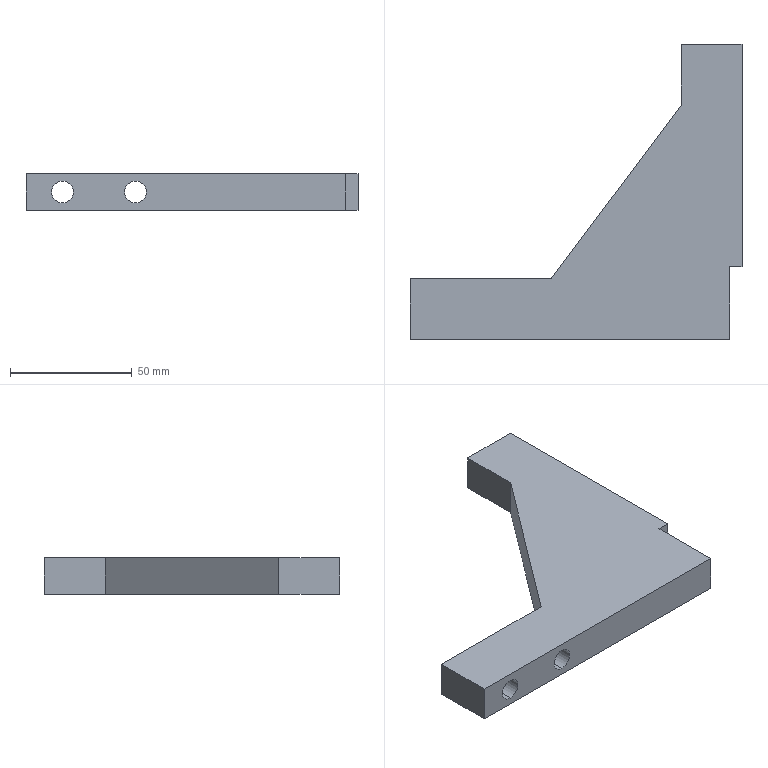Part | STEP file | 07-05 triangular support bracket | 1 solid | 27 faces | box 136.5 x 121.3 x 15 mm | volume 109879 mm3 | plane 11 | cylinder 10 | cone 6 | commonest cylinder face diameters 4.2 x6 9 x4
STEP:
#1=CARTESIAN_POINT('',(52.988,50.65,7.5));
#2=VERTEX_POINT('',#1);
#3=CARTESIAN_POINT('',(54.25,50.65,5.4));
#4=VERTEX_POINT('',#3);
#5=CARTESIAN_POINT('',(54.25,50.65,5.4));
#6=DIRECTION('',(0.515,0.,-0.8572));
#7=VECTOR('',#6,1000.);
#8=LINE('',#5,#7);
#9=EDGE_CURVE('',#2,#4,#8,.T.);
#10=ORIENTED_EDGE('',*,*,#9,.F.);
#11=CARTESIAN_POINT('',(54.25,50.65,9.6));
#12=VERTEX_POINT('',#11);
#13=CARTESIAN_POINT('',(54.25,50.65,9.6));
#14=DIRECTION('',(0.515,0.,0.8572));
#15=VECTOR('',#14,1000.);
#16=LINE('',#13,#15);
#17=EDGE_CURVE('',#2,#12,#16,.T.);
#18=ORIENTED_EDGE('',*,*,#17,.T.);
#19=CARTESIAN_POINT('',(54.25,50.65,7.5));
#20=DIRECTION('',(1.,0.,0.));
#21=DIRECTION('',(0.,0.,-1.));
#22=AXIS2_PLACEMENT_3D('',#19,#20,#21);
#23=CIRCLE('',#22,2.1);
#24=EDGE_CURVE('',#12,#4,#23,.T.);
#25=ORIENTED_EDGE('',*,*,#24,.T.);
#26=EDGE_LOOP('',(#10,#18,#25));
#27=FACE_OUTER_BOUND('',#26,.T.);
#28=CARTESIAN_POINT('',(54.25,50.65,7.5));
#29=DIRECTION('',(1.,0.,0.));
#30=DIRECTION('',(0.,0.,-1.));
#31=AXIS2_PLACEMENT_3D('',#28,#29,#30);
#32=CONICAL_SURFACE('',#31,2.1,1.03);
#33=ADVANCED_FACE('',(#27),#32,.F.);
#34=ORIENTED_EDGE('',*,*,#24,.F.);
#35=CARTESIAN_POINT('',(68.25,50.65,9.6));
#36=VERTEX_POINT('',#35);
#37=CARTESIAN_POINT('',(68.25,50.65,9.6));
#38=DIRECTION('',(1.,0.,0.));
#39=VECTOR('',#38,1000.);
#40=LINE('',#37,#39);
#41=EDGE_CURVE('',#12,#36,#40,.T.);
#42=ORIENTED_EDGE('',*,*,#41,.T.);
#43=CARTESIAN_POINT('',(68.25,50.65,5.4));
#44=VERTEX_POINT('',#43);
#45=CARTESIAN_POINT('',(68.25,50.65,7.5));
#46=DIRECTION('',(1.,0.,0.));
#47=DIRECTION('',(0.,0.,-1.));
#48=AXIS2_PLACEMENT_3D('',#45,#46,#47);
#49=CIRCLE('',#48,2.1);
#50=EDGE_CURVE('',#36,#44,#49,.T.);
#51=ORIENTED_EDGE('',*,*,#50,.T.);
#52=CARTESIAN_POINT('',(68.25,50.65,5.4));
#53=DIRECTION('',(1.,0.,0.));
#54=VECTOR('',#53,1000.);
#55=LINE('',#52,#54);
#56=EDGE_CURVE('',#4,#44,#55,.T.);
#57=ORIENTED_EDGE('',*,*,#56,.F.);
#58=EDGE_LOOP('',(#34,#42,#51,#57));
#59=FACE_OUTER_BOUND('',#58,.T.);
#60=CARTESIAN_POINT('',(68.25,50.65,7.5));
#61=DIRECTION('',(1.,0.,0.));
#62=DIRECTION('',(0.,0.,-1.));
#63=AXIS2_PLACEMENT_3D('',#60,#61,#62);
#64=CYLINDRICAL_SURFACE('',#63,2.1);
#65=ADVANCED_FACE('',(#59),#64,.F.);
#66=CARTESIAN_POINT('',(54.25,15.65,9.6));
#67=VERTEX_POINT('',#66);
#68=CARTESIAN_POINT('',(54.25,15.65,5.4));
#69=VERTEX_POINT('',#68);
#70=CARTESIAN_POINT('',(54.25,15.65,7.5));
#71=DIRECTION('',(1.,0.,0.));
#72=DIRECTION('',(0.,0.,-1.));
#73=AXIS2_PLACEMENT_3D('',#70,#71,#72);
#74=CIRCLE('',#73,2.1);
#75=EDGE_CURVE('',#67,#69,#74,.T.);
#76=ORIENTED_EDGE('',*,*,#75,.F.);
#77=CARTESIAN_POINT('',(68.25,15.65,9.6));
#78=VERTEX_POINT('',#77);
#79=CARTESIAN_POINT('',(68.25,15.65,9.6));
#80=DIRECTION('',(1.,0.,0.));
#81=VECTOR('',#80,1000.);
#82=LINE('',#79,#81);
#83=EDGE_CURVE('',#67,#78,#82,.T.);
#84=ORIENTED_EDGE('',*,*,#83,.T.);
#85=CARTESIAN_POINT('',(68.25,15.65,5.4));
#86=VERTEX_POINT('',#85);
#87=CARTESIAN_POINT('',(68.25,15.65,7.5));
#88=DIRECTION('',(1.,0.,0.));
#89=DIRECTION('',(0.,0.,-1.));
#90=AXIS2_PLACEMENT_3D('',#87,#88,#89);
#91=CIRCLE('',#90,2.1);
#92=EDGE_CURVE('',#78,#86,#91,.T.);
#93=ORIENTED_EDGE('',*,*,#92,.T.);
#94=CARTESIAN_POINT('',(68.25,15.65,5.4));
#95=DIRECTION('',(1.,0.,0.));
#96=VECTOR('',#95,1000.);
#97=LINE('',#94,#96);
#98=EDGE_CURVE('',#69,#86,#97,.T.);
#99=ORIENTED_EDGE('',*,*,#98,.F.);
#100=EDGE_LOOP('',(#76,#84,#93,#99));
#101=FACE_OUTER_BOUND('',#100,.T.);
#102=CARTESIAN_POINT('',(68.25,15.65,7.5));
#103=DIRECTION('',(1.,0.,0.));
#104=DIRECTION('',(0.,0.,-1.));
#105=AXIS2_PLACEMENT_3D('',#102,#103,#104);
#106=CYLINDRICAL_SURFACE('',#105,2.1);
#107=ADVANCED_FACE('',(#101),#106,.F.);
#108=CARTESIAN_POINT('',(52.988,15.65,7.5));
#109=VERTEX_POINT('',#108);
#110=CARTESIAN_POINT('',(54.25,15.65,5.4));
#111=DIRECTION('',(0.515,0.,-0.8572));
#112=VECTOR('',#111,1000.);
#113=LINE('',#110,#112);
#114=EDGE_CURVE('',#109,#69,#113,.T.);
#115=ORIENTED_EDGE('',*,*,#114,.F.);
#116=CARTESIAN_POINT('',(54.25,15.65,9.6));
#117=DIRECTION('',(0.515,0.,0.8572));
#118=VECTOR('',#117,1000.);
#119=LINE('',#116,#118);
#120=EDGE_CURVE('',#109,#67,#119,.T.);
#121=ORIENTED_EDGE('',*,*,#120,.T.);
#122=ORIENTED_EDGE('',*,*,#75,.T.);
#123=EDGE_LOOP('',(#115,#121,#122));
#124=FACE_OUTER_BOUND('',#123,.T.);
#125=CARTESIAN_POINT('',(54.25,15.65,7.5));
#126=DIRECTION('',(1.,0.,0.));
#127=DIRECTION('',(0.,0.,-1.));
#128=AXIS2_PLACEMENT_3D('',#125,#126,#127);
#129=CONICAL_SURFACE('',#128,2.1,1.03);
#130=ADVANCED_FACE('',(#124),#129,.F.);
#131=CARTESIAN_POINT('',(54.25,-19.35,9.6));
#132=VERTEX_POINT('',#131);
#133=CARTESIAN_POINT('',(54.25,-19.35,5.4));
#134=VERTEX_POINT('',#133);
#135=CARTESIAN_POINT('',(54.25,-19.35,7.5));
#136=DIRECTION('',(1.,0.,0.));
#137=DIRECTION('',(0.,0.,-1.));
#138=AXIS2_PLACEMENT_3D('',#135,#136,#137);
#139=CIRCLE('',#138,2.1);
#140=EDGE_CURVE('',#132,#134,#139,.T.);
#141=ORIENTED_EDGE('',*,*,#140,.F.);
#142=CARTESIAN_POINT('',(68.25,-19.35,9.6));
#143=VERTEX_POINT('',#142);
#144=CARTESIAN_POINT('',(68.25,-19.35,9.6));
#145=DIRECTION('',(1.,0.,0.));
#146=VECTOR('',#145,1000.);
#147=LINE('',#144,#146);
#148=EDGE_CURVE('',#132,#143,#147,.T.);
#149=ORIENTED_EDGE('',*,*,#148,.T.);
#150=CARTESIAN_POINT('',(68.25,-19.35,5.4));
#151=VERTEX_POINT('',#150);
#152=CARTESIAN_POINT('',(68.25,-19.35,7.5));
#153=DIRECTION('',(1.,0.,0.));
#154=DIRECTION('',(0.,0.,-1.));
#155=AXIS2_PLACEMENT_3D('',#152,#153,#154);
#156=CIRCLE('',#155,2.1);
#157=EDGE_CURVE('',#143,#151,#156,.T.);
#158=ORIENTED_EDGE('',*,*,#157,.T.);
#159=CARTESIAN_POINT('',(68.25,-19.35,5.4));
#160=DIRECTION('',(1.,0.,0.));
#161=VECTOR('',#160,1000.);
#162=LINE('',#159,#161);
#163=EDGE_CURVE('',#134,#151,#162,.T.);
#164=ORIENTED_EDGE('',*,*,#163,.F.);
#165=EDGE_LOOP('',(#141,#149,#158,#164));
#166=FACE_OUTER_BOUND('',#165,.T.);
#167=CARTESIAN_POINT('',(68.25,-19.35,7.5));
#168=DIRECTION('',(1.,0.,0.));
#169=DIRECTION('',(0.,0.,-1.));
#170=AXIS2_PLACEMENT_3D('',#167,#168,#169);
#171=CYLINDRICAL_SURFACE('',#170,2.1);
#172=ADVANCED_FACE('',(#166),#171,.F.);
#173=CARTESIAN_POINT('',(52.988,-19.35,7.5));
#174=VERTEX_POINT('',#173);
#175=CARTESIAN_POINT('',(54.25,-19.35,5.4));
#176=DIRECTION('',(0.515,0.,-0.8572));
#177=VECTOR('',#176,1000.);
#178=LINE('',#175,#177);
#179=EDGE_CURVE('',#174,#134,#178,.T.);
#180=ORIENTED_EDGE('',*,*,#179,.F.);
#181=CARTESIAN_POINT('',(54.25,-19.35,9.6));
#182=DIRECTION('',(0.515,0.,0.8572));
#183=VECTOR('',#182,1000.);
#184=LINE('',#181,#183);
#185=EDGE_CURVE('',#174,#132,#184,.T.);
#186=ORIENTED_EDGE('',*,*,#185,.T.);
#187=ORIENTED_EDGE('',*,*,#140,.T.);
#188=EDGE_LOOP('',(#180,#186,#187));
#189=FACE_OUTER_BOUND('',#188,.T.);
#190=CARTESIAN_POINT('',(54.25,-19.35,7.5));
#191=DIRECTION('',(1.,0.,0.));
#192=DIRECTION('',(0.,0.,-1.));
#193=AXIS2_PLACEMENT_3D('',#190,#191,#192);
#194=CONICAL_SURFACE('',#193,2.1,1.03);
#195=ADVANCED_FACE('',(#189),#194,.F.);
#196=CARTESIAN_POINT('',(-23.25,-60.65,3.));
#197=VERTEX_POINT('',#196);
#198=CARTESIAN_POINT('',(-23.25,-60.65,12.));
#199=VERTEX_POINT('',#198);
#200=CARTESIAN_POINT('',(-23.25,-60.65,7.5));
#201=DIRECTION('',(0.,1.,0.));
#202=DIRECTION('',(0.,0.,1.));
#203=AXIS2_PLACEMENT_3D('',#200,#201,#202);
#204=CIRCLE('',#203,4.5);
#205=EDGE_CURVE('',#197,#199,#204,.T.);
#206=ORIENTED_EDGE('',*,*,#205,.F.);
#207=CARTESIAN_POINT('',(-23.25,-35.65,3.));
#208=VERTEX_POINT('',#207);
#209=CARTESIAN_POINT('',(-23.25,-65.65,3.));
#210=DIRECTION('',(0.,1.,0.));
#211=VECTOR('',#210,1000.);
#212=LINE('',#209,#211);
#213=EDGE_CURVE('',#197,#208,#212,.T.);
#214=ORIENTED_EDGE('',*,*,#213,.T.);
#215=CARTESIAN_POINT('',(-23.25,-35.65,12.));
#216=VERTEX_POINT('',#215);
#217=CARTESIAN_POINT('',(-23.25,-35.65,7.5));
#218=DIRECTION('',(0.,-1.,0.));
#219=DIRECTION('',(0.,0.,-1.));
#220=AXIS2_PLACEMENT_3D('',#217,#218,#219);
#221=CIRCLE('',#220,4.5);
#222=EDGE_CURVE('',#216,#208,#221,.T.);
#223=ORIENTED_EDGE('',*,*,#222,.F.);
#224=CARTESIAN_POINT('',(-23.25,-65.65,12.));
#225=DIRECTION('',(0.,1.,0.));
#226=VECTOR('',#225,1000.);
#227=LINE('',#224,#226);
#228=EDGE_CURVE('',#199,#216,#227,.T.);
#229=ORIENTED_EDGE('',*,*,#228,.F.);
#230=EDGE_LOOP('',(#206,#214,#223,#229));
#231=FACE_OUTER_BOUND('',#230,.T.);
#232=CARTESIAN_POINT('',(-23.25,-65.65,7.5));
#233=DIRECTION('',(0.,1.,0.));
#234=DIRECTION('',(0.,0.,1.));
#235=AXIS2_PLACEMENT_3D('',#232,#233,#234);
#236=CYLINDRICAL_SURFACE('',#235,4.5);
#237=ADVANCED_FACE('',(#231),#236,.F.);
#238=CARTESIAN_POINT('',(-53.25,-60.65,3.));
#239=VERTEX_POINT('',#238);
#240=CARTESIAN_POINT('',(-53.25,-60.65,12.));
#241=VERTEX_POINT('',#240);
#242=CARTESIAN_POINT('',(-53.25,-60.65,7.5));
#243=DIRECTION('',(0.,1.,0.));
#244=DIRECTION('',(0.,0.,1.));
#245=AXIS2_PLACEMENT_3D('',#242,#243,#244);
#246=CIRCLE('',#245,4.5);
#247=EDGE_CURVE('',#239,#241,#246,.T.);
#248=ORIENTED_EDGE('',*,*,#247,.F.);
#249=CARTESIAN_POINT('',(-53.25,-35.65,3.));
#250=VERTEX_POINT('',#249);
#251=CARTESIAN_POINT('',(-53.25,-65.65,3.));
#252=DIRECTION('',(0.,1.,0.));
#253=VECTOR('',#252,1000.);
#254=LINE('',#251,#253);
#255=EDGE_CURVE('',#239,#250,#254,.T.);
#256=ORIENTED_EDGE('',*,*,#255,.T.);
#257=CARTESIAN_POINT('',(-53.25,-35.65,12.));
#258=VERTEX_POINT('',#257);
#259=CARTESIAN_POINT('',(-53.25,-35.65,7.5));
#260=DIRECTION('',(0.,-1.,0.));
#261=DIRECTION('',(0.,0.,-1.));
#262=AXIS2_PLACEMENT_3D('',#259,#260,#261);
#263=CIRCLE('',#262,4.5);
#264=EDGE_CURVE('',#258,#250,#263,.T.);
#265=ORIENTED_EDGE('',*,*,#264,.F.);
#266=CARTESIAN_POINT('',(-53.25,-65.65,12.));
#267=DIRECTION('',(0.,1.,0.));
#268=VECTOR('',#267,1000.);
#269=LINE('',#266,#268);
#270=EDGE_CURVE('',#241,#258,#269,.T.);
#271=ORIENTED_EDGE('',*,*,#270,.F.);
#272=EDGE_LOOP('',(#248,#256,#265,#271));
#273=FACE_OUTER_BOUND('',#272,.T.);
#274=CARTESIAN_POINT('',(-53.25,-65.65,7.5));
#275=DIRECTION('',(0.,1.,0.));
#276=DIRECTION('',(0.,0.,1.));
#277=AXIS2_PLACEMENT_3D('',#274,#275,#276);
#278=CYLINDRICAL_SURFACE('',#277,4.5);
#279=ADVANCED_FACE('',(#273),#278,.F.);
#280=CARTESIAN_POINT('',(68.25,15.65,7.5));
#281=DIRECTION('',(1.,0.,0.));
#282=DIRECTION('',(0.,0.,-1.));
#283=AXIS2_PLACEMENT_3D('',#280,#281,#282);
#284=CIRCLE('',#283,2.1);
#285=EDGE_CURVE('',#86,#78,#284,.T.);
#286=ORIENTED_EDGE('',*,*,#285,.F.);
#287=ORIENTED_EDGE('',*,*,#92,.F.);
#288=EDGE_LOOP('',(#286,#287));
#289=FACE_BOUND('',#288,.T.);
#290=CARTESIAN_POINT('',(68.25,-19.35,7.5));
#291=DIRECTION('',(1.,0.,0.));
#292=DIRECTION('',(0.,0.,-1.));
#293=AXIS2_PLACEMENT_3D('',#290,#291,#292);
#294=CIRCLE('',#293,2.1);
#295=EDGE_CURVE('',#151,#143,#294,.T.);
#296=ORIENTED_EDGE('',*,*,#295,.F.);
#297=ORIENTED_EDGE('',*,*,#157,.F.);
#298=EDGE_LOOP('',(#296,#297));
#299=FACE_BOUND('',#298,.T.);
#300=CARTESIAN_POINT('',(68.25,-30.65,15.));
#301=VERTEX_POINT('',#300);
#302=CARTESIAN_POINT('',(68.25,60.65,15.));
#303=VERTEX_POINT('',#302);
#304=CARTESIAN_POINT('',(68.25,-60.65,15.));
#305=DIRECTION('',(0.,1.,0.));
#306=VECTOR('',#305,1000.);
#307=LINE('',#304,#306);
#308=EDGE_CURVE('',#301,#303,#307,.T.);
#309=ORIENTED_EDGE('',*,*,#308,.F.);
#310=CARTESIAN_POINT('',(68.25,-30.65,0.));
#311=VERTEX_POINT('',#310);
#312=CARTESIAN_POINT('',(68.25,-30.65,-83.));
#313=DIRECTION('',(0.,0.,1.));
#314=VECTOR('',#313,1000.);
#315=LINE('',#312,#314);
#316=EDGE_CURVE('',#311,#301,#315,.T.);
#317=ORIENTED_EDGE('',*,*,#316,.F.);
#318=CARTESIAN_POINT('',(68.25,60.65,0.));
#319=VERTEX_POINT('',#318);
#320=CARTESIAN_POINT('',(68.25,-60.65,0.));
#321=DIRECTION('',(0.,1.,0.));
#322=VECTOR('',#321,1000.);
#323=LINE('',#320,#322);
#324=EDGE_CURVE('',#311,#319,#323,.T.);
#325=ORIENTED_EDGE('',*,*,#324,.T.);
#326=CARTESIAN_POINT('',(68.25,60.65,15.));
#327=DIRECTION('',(0.,0.,-1.));
#328=VECTOR('',#327,1000.);
#329=LINE('',#326,#328);
#330=EDGE_CURVE('',#303,#319,#329,.T.);
#331=ORIENTED_EDGE('',*,*,#330,.F.);
#332=EDGE_LOOP('',(#309,#317,#325,#331));
#333=FACE_OUTER_BOUND('',#332,.T.);
#334=CARTESIAN_POINT('',(68.25,50.65,7.5));
#335=DIRECTION('',(1.,0.,0.));
#336=DIRECTION('',(0.,0.,-1.));
#337=AXIS2_PLACEMENT_3D('',#334,#335,#336);
#338=CIRCLE('',#337,2.1);
#339=EDGE_CURVE('',#44,#36,#338,.T.);
#340=ORIENTED_EDGE('',*,*,#339,.F.);
#341=ORIENTED_EDGE('',*,*,#50,.F.);
#342=EDGE_LOOP('',(#340,#341));
#343=FACE_BOUND('',#342,.T.);
#344=CARTESIAN_POINT('',(68.25,-60.65,15.));
#345=DIRECTION('',(-1.,0.,0.));
#346=DIRECTION('',(0.,0.,1.));
#347=AXIS2_PLACEMENT_3D('',#344,#345,#346);
#348=PLANE('',#347);
#349=ADVANCED_FACE('',(#289,#299,#333,#343),#348,.F.);
#350=CARTESIAN_POINT('',(43.25,60.65,0.));
#351=VERTEX_POINT('',#350);
#352=CARTESIAN_POINT('',(-68.25,60.65,0.));
#353=DIRECTION('',(-1.,0.,0.));
#354=VECTOR('',#353,1000.);
#355=LINE('',#352,#354);
#356=EDGE_CURVE('',#319,#351,#355,.T.);
#357=ORIENTED_EDGE('',*,*,#356,.T.);
#358=CARTESIAN_POINT('',(43.25,60.65,15.));
#359=VERTEX_POINT('',#358);
#360=CARTESIAN_POINT('',(43.25,60.65,-33.));
#361=DIRECTION('',(0.,0.,1.));
#362=VECTOR('',#361,1000.);
#363=LINE('',#360,#362);
#364=EDGE_CURVE('',#351,#359,#363,.T.);
#365=ORIENTED_EDGE('',*,*,#364,.T.);
#366=CARTESIAN_POINT('',(-68.25,60.65,15.));
#367=DIRECTION('',(-1.,0.,0.));
#368=VECTOR('',#367,1000.);
#369=LINE('',#366,#368);
#370=EDGE_CURVE('',#303,#359,#369,.T.);
#371=ORIENTED_EDGE('',*,*,#370,.F.);
#372=ORIENTED_EDGE('',*,*,#330,.T.);
#373=EDGE_LOOP('',(#357,#365,#371,#372));
#374=FACE_OUTER_BOUND('',#373,.T.);
#375=CARTESIAN_POINT('',(-68.25,60.65,15.));
#376=DIRECTION('',(0.,-1.,0.));
#377=DIRECTION('',(0.,0.,-1.));
#378=AXIS2_PLACEMENT_3D('',#375,#376,#377);
#379=PLANE('',#378);
#380=ADVANCED_FACE('',(#374),#379,.F.);
#381=CARTESIAN_POINT('',(-68.25,-35.65,15.));
#382=VERTEX_POINT('',#381);
#383=CARTESIAN_POINT('',(-68.25,-60.65,15.));
#384=VERTEX_POINT('',#383);
#385=CARTESIAN_POINT('',(-68.25,-60.65,15.));
#386=DIRECTION('',(0.,-1.,0.));
#387=VECTOR('',#386,1000.);
#388=LINE('',#385,#387);
#389=EDGE_CURVE('',#382,#384,#388,.T.);
#390=ORIENTED_EDGE('',*,*,#389,.F.);
#391=CARTESIAN_POINT('',(-68.25,-35.65,0.));
#392=VERTEX_POINT('',#391);
#393=CARTESIAN_POINT('',(-68.25,-35.65,-33.));
#394=DIRECTION('',(0.,0.,1.));
#395=VECTOR('',#394,1000.);
#396=LINE('',#393,#395);
#397=EDGE_CURVE('',#392,#382,#396,.T.);
#398=ORIENTED_EDGE('',*,*,#397,.F.);
#399=CARTESIAN_POINT('',(-68.25,-60.65,0.));
#400=VERTEX_POINT('',#399);
#401=CARTESIAN_POINT('',(-68.25,-60.65,0.));
#402=DIRECTION('',(0.,-1.,0.));
#403=VECTOR('',#402,1000.);
#404=LINE('',#401,#403);
#405=EDGE_CURVE('',#392,#400,#404,.T.);
#406=ORIENTED_EDGE('',*,*,#405,.T.);
#407=CARTESIAN_POINT('',(-68.25,-60.65,15.));
#408=DIRECTION('',(0.,0.,-1.));
#409=VECTOR('',#408,1000.);
#410=LINE('',#407,#409);
#411=EDGE_CURVE('',#384,#400,#410,.T.);
#412=ORIENTED_EDGE('',*,*,#411,.F.);
#413=EDGE_LOOP('',(#390,#398,#406,#412));
#414=FACE_OUTER_BOUND('',#413,.T.);
#415=CARTESIAN_POINT('',(-68.25,-60.65,15.));
#416=DIRECTION('',(1.,0.,0.));
#417=DIRECTION('',(0.,0.,-1.));
#418=AXIS2_PLACEMENT_3D('',#415,#416,#417);
#419=PLANE('',#418);
#420=ADVANCED_FACE('',(#414),#419,.F.);
#421=CARTESIAN_POINT('',(-23.25,-60.65,7.5));
#422=DIRECTION('',(0.,1.,0.));
#423=DIRECTION('',(0.,0.,1.));
#424=AXIS2_PLACEMENT_3D('',#421,#422,#423);
#425=CIRCLE('',#424,4.5);
#426=EDGE_CURVE('',#199,#197,#425,.T.);
#427=ORIENTED_EDGE('',*,*,#426,.T.);
#428=ORIENTED_EDGE('',*,*,#205,.T.);
#429=EDGE_LOOP('',(#427,#428));
#430=FACE_BOUND('',#429,.T.);
#431=CARTESIAN_POINT('',(-53.25,-60.65,7.5));
#432=DIRECTION('',(0.,1.,0.));
#433=DIRECTION('',(0.,0.,1.));
#434=AXIS2_PLACEMENT_3D('',#431,#432,#433);
#435=CIRCLE('',#434,4.5);
#436=EDGE_CURVE('',#241,#239,#435,.T.);
#437=ORIENTED_EDGE('',*,*,#436,.T.);
#438=ORIENTED_EDGE('',*,*,#247,.T.);
#439=EDGE_LOOP('',(#437,#438));
#440=FACE_BOUND('',#439,.T.);
#441=CARTESIAN_POINT('',(63.25,-60.65,0.));
#442=VERTEX_POINT('',#441);
#443=CARTESIAN_POINT('',(-68.25,-60.65,0.));
#444=DIRECTION('',(1.,0.,0.));
#445=VECTOR('',#444,1000.);
#446=LINE('',#443,#445);
#447=EDGE_CURVE('',#400,#442,#446,.T.);
#448=ORIENTED_EDGE('',*,*,#447,.T.);
#449=CARTESIAN_POINT('',(63.25,-60.65,15.));
#450=VERTEX_POINT('',#449);
#451=CARTESIAN_POINT('',(63.25,-60.65,-83.));
#452=DIRECTION('',(0.,0.,1.));
#453=VECTOR('',#452,1000.);
#454=LINE('',#451,#453);
#455=EDGE_CURVE('',#442,#450,#454,.T.);
#456=ORIENTED_EDGE('',*,*,#455,.T.);
#457=CARTESIAN_POINT('',(-68.25,-60.65,15.));
#458=DIRECTION('',(1.,0.,0.));
#459=VECTOR('',#458,1000.);
#460=LINE('',#457,#459);
#461=EDGE_CURVE('',#384,#450,#460,.T.);
#462=ORIENTED_EDGE('',*,*,#461,.F.);
#463=ORIENTED_EDGE('',*,*,#411,.T.);
#464=EDGE_LOOP('',(#448,#456,#462,#463));
#465=FACE_OUTER_BOUND('',#464,.T.);
#466=CARTESIAN_POINT('',(-68.25,-60.65,15.));
#467=DIRECTION('',(0.,1.,0.));
#468=DIRECTION('',(0.,0.,1.));
#469=AXIS2_PLACEMENT_3D('',#466,#467,#468);
#470=PLANE('',#469);
#471=ADVANCED_FACE('',(#430,#440,#465),#470,.F.);
#472=ORIENTED_EDGE('',*,*,#461,.T.);
#473=CARTESIAN_POINT('',(63.25,-30.65,15.));
#474=VERTEX_POINT('',#473);
#475=CARTESIAN_POINT('',(63.25,-60.65,15.));
#476=DIRECTION('',(0.,-1.,0.));
#477=VECTOR('',#476,1000.);
#478=LINE('',#475,#477);
#479=EDGE_CURVE('',#474,#450,#478,.T.);
#480=ORIENTED_EDGE('',*,*,#479,.F.);
#481=CARTESIAN_POINT('',(68.25,-30.65,15.));
#482=DIRECTION('',(-1.,0.,0.));
#483=VECTOR('',#482,1000.);
#484=LINE('',#481,#483);
#485=EDGE_CURVE('',#301,#474,#484,.T.);
#486=ORIENTED_EDGE('',*,*,#485,.F.);
#487=ORIENTED_EDGE('',*,*,#308,.T.);
#488=ORIENTED_EDGE('',*,*,#370,.T.);
#489=CARTESIAN_POINT('',(43.25,35.65,15.));
#490=VERTEX_POINT('',#489);
#491=CARTESIAN_POINT('',(43.25,60.65,15.));
#492=DIRECTION('',(0.,1.,0.));
#493=VECTOR('',#492,1000.);
#494=LINE('',#491,#493);
#495=EDGE_CURVE('',#490,#359,#494,.T.);
#496=ORIENTED_EDGE('',*,*,#495,.F.);
#497=CARTESIAN_POINT('',(-10.25,-35.65,15.));
#498=VERTEX_POINT('',#497);
#499=CARTESIAN_POINT('',(43.25,35.65,15.));
#500=DIRECTION('',(0.6002,0.7999,0.));
#501=VECTOR('',#500,1000.);
#502=LINE('',#499,#501);
#503=EDGE_CURVE('',#498,#490,#502,.T.);
#504=ORIENTED_EDGE('',*,*,#503,.F.);
#505=CARTESIAN_POINT('',(-68.25,-35.65,15.));
#506=DIRECTION('',(1.,0.,0.));
#507=VECTOR('',#506,1000.);
#508=LINE('',#505,#507);
#509=EDGE_CURVE('',#382,#498,#508,.T.);
#510=ORIENTED_EDGE('',*,*,#509,.F.);
#511=ORIENTED_EDGE('',*,*,#389,.T.);
#512=EDGE_LOOP('',(#472,#480,#486,#487,#488,#496,#504,#510,#511));
#513=FACE_OUTER_BOUND('',#512,.T.);
#514=CARTESIAN_POINT('',(68.25,60.65,15.));
#515=DIRECTION('',(0.,0.,-1.));
#516=DIRECTION('',(-1.,0.,0.));
#517=AXIS2_PLACEMENT_3D('',#514,#515,#516);
#518=PLANE('',#517);
#519=ADVANCED_FACE('',(#513),#518,.F.);
#520=CARTESIAN_POINT('',(63.25,-30.65,0.));
#521=VERTEX_POINT('',#520);
#522=CARTESIAN_POINT('',(63.25,60.65,0.));
#523=DIRECTION('',(0.,1.,0.));
#524=VECTOR('',#523,1000.);
#525=LINE('',#522,#524);
#526=EDGE_CURVE('',#442,#521,#525,.T.);
#527=ORIENTED_EDGE('',*,*,#526,.F.);
#528=ORIENTED_EDGE('',*,*,#447,.F.);
#529=ORIENTED_EDGE('',*,*,#405,.F.);
#530=CARTESIAN_POINT('',(-10.25,-35.65,0.));
#531=VERTEX_POINT('',#530);
#532=CARTESIAN_POINT('',(68.25,-35.65,0.));
#533=DIRECTION('',(-1.,0.,0.));
#534=VECTOR('',#533,1000.);
#535=LINE('',#532,#534);
#536=EDGE_CURVE('',#531,#392,#535,.T.);
#537=ORIENTED_EDGE('',*,*,#536,.F.);
#538=CARTESIAN_POINT('',(43.25,35.65,0.));
#539=VERTEX_POINT('',#538);
#540=CARTESIAN_POINT('',(64.257,63.646,0.));
#541=DIRECTION('',(-0.6002,-0.7999,0.));
#542=VECTOR('',#541,1000.);
#543=LINE('',#540,#542);
#544=EDGE_CURVE('',#539,#531,#543,.T.);
#545=ORIENTED_EDGE('',*,*,#544,.F.);
#546=CARTESIAN_POINT('',(43.25,60.65,0.));
#547=DIRECTION('',(0.,-1.,0.));
#548=VECTOR('',#547,1000.);
#549=LINE('',#546,#548);
#550=EDGE_CURVE('',#351,#539,#549,.T.);
#551=ORIENTED_EDGE('',*,*,#550,.F.);
#552=ORIENTED_EDGE('',*,*,#356,.F.);
#553=ORIENTED_EDGE('',*,*,#324,.F.);
#554=CARTESIAN_POINT('',(68.25,-30.65,0.));
#555=DIRECTION('',(1.,0.,0.));
#556=VECTOR('',#555,1000.);
#557=LINE('',#554,#556);
#558=EDGE_CURVE('',#521,#311,#557,.T.);
#559=ORIENTED_EDGE('',*,*,#558,.F.);
#560=EDGE_LOOP('',(#527,#528,#529,#537,#545,#551,#552,#553,#559));
#561=FACE_OUTER_BOUND('',#560,.T.);
#562=CARTESIAN_POINT('',(68.25,60.65,0.));
#563=DIRECTION('',(0.,0.,-1.));
#564=DIRECTION('',(-1.,0.,0.));
#565=AXIS2_PLACEMENT_3D('',#562,#563,#564);
#566=PLANE('',#565);
#567=ADVANCED_FACE('',(#561),#566,.T.);
#568=ORIENTED_EDGE('',*,*,#550,.T.);
#569=CARTESIAN_POINT('',(43.25,35.65,-33.));
#570=DIRECTION('',(0.,0.,1.));
#571=VECTOR('',#570,1000.);
#572=LINE('',#569,#571);
#573=EDGE_CURVE('',#539,#490,#572,.T.);
#574=ORIENTED_EDGE('',*,*,#573,.T.);
#575=ORIENTED_EDGE('',*,*,#495,.T.);
#576=ORIENTED_EDGE('',*,*,#364,.F.);
#577=EDGE_LOOP('',(#568,#574,#575,#576));
#578=FACE_OUTER_BOUND('',#577,.T.);
#579=CARTESIAN_POINT('',(43.25,60.65,-33.));
#580=DIRECTION('',(1.,0.,0.));
#581=DIRECTION('',(0.,1.,0.));
#582=AXIS2_PLACEMENT_3D('',#579,#580,#581);
#583=PLANE('',#582);
#584=ADVANCED_FACE('',(#578),#583,.F.);
#585=ORIENTED_EDGE('',*,*,#544,.T.);
#586=CARTESIAN_POINT('',(-10.25,-35.65,-33.));
#587=DIRECTION('',(0.,0.,1.));
#588=VECTOR('',#587,1000.);
#589=LINE('',#586,#588);
#590=EDGE_CURVE('',#531,#498,#589,.T.);
#591=ORIENTED_EDGE('',*,*,#590,.T.);
#592=ORIENTED_EDGE('',*,*,#503,.T.);
#593=ORIENTED_EDGE('',*,*,#573,.F.);
#594=EDGE_LOOP('',(#585,#591,#592,#593));
#595=FACE_OUTER_BOUND('',#594,.T.);
#596=CARTESIAN_POINT('',(43.25,35.65,-33.));
#597=DIRECTION('',(0.7999,-0.6002,0.));
#598=DIRECTION('',(0.6002,0.7999,0.));
#599=AXIS2_PLACEMENT_3D('',#596,#597,#598);
#600=PLANE('',#599);
#601=ADVANCED_FACE('',(#595),#600,.F.);
#602=ORIENTED_EDGE('',*,*,#222,.T.);
#603=CARTESIAN_POINT('',(-23.25,-35.65,7.5));
#604=DIRECTION('',(0.,-1.,0.));
#605=DIRECTION('',(0.,0.,-1.));
#606=AXIS2_PLACEMENT_3D('',#603,#604,#605);
#607=CIRCLE('',#606,4.5);
#608=EDGE_CURVE('',#208,#216,#607,.T.);
#609=ORIENTED_EDGE('',*,*,#608,.T.);
#610=EDGE_LOOP('',(#602,#609));
#611=FACE_BOUND('',#610,.T.);
#612=ORIENTED_EDGE('',*,*,#264,.T.);
#613=CARTESIAN_POINT('',(-53.25,-35.65,7.5));
#614=DIRECTION('',(0.,-1.,0.));
#615=DIRECTION('',(0.,0.,-1.));
#616=AXIS2_PLACEMENT_3D('',#613,#614,#615);
#617=CIRCLE('',#616,4.5);
#618=EDGE_CURVE('',#250,#258,#617,.T.);
#619=ORIENTED_EDGE('',*,*,#618,.T.);
#620=EDGE_LOOP('',(#612,#619));
#621=FACE_BOUND('',#620,.T.);
#622=ORIENTED_EDGE('',*,*,#536,.T.);
#623=ORIENTED_EDGE('',*,*,#397,.T.);
#624=ORIENTED_EDGE('',*,*,#509,.T.);
#625=ORIENTED_EDGE('',*,*,#590,.F.);
#626=EDGE_LOOP('',(#622,#623,#624,#625));
#627=FACE_OUTER_BOUND('',#626,.T.);
#628=CARTESIAN_POINT('',(-68.25,-35.65,-33.));
#629=DIRECTION('',(0.,-1.,0.));
#630=DIRECTION('',(0.,0.,-1.));
#631=AXIS2_PLACEMENT_3D('',#628,#629,#630);
#632=PLANE('',#631);
#633=ADVANCED_FACE('',(#611,#621,#627),#632,.F.);
#634=ORIENTED_EDGE('',*,*,#255,.F.);
#635=ORIENTED_EDGE('',*,*,#436,.F.);
#636=ORIENTED_EDGE('',*,*,#270,.T.);
#637=ORIENTED_EDGE('',*,*,#618,.F.);
#638=EDGE_LOOP('',(#634,#635,#636,#637));
#639=FACE_OUTER_BOUND('',#638,.T.);
#640=CARTESIAN_POINT('',(-53.25,-65.65,7.5));
#641=DIRECTION('',(0.,1.,0.));
#642=DIRECTION('',(0.,0.,1.));
#643=AXIS2_PLACEMENT_3D('',#640,#641,#642);
#644=CYLINDRICAL_SURFACE('',#643,4.5);
#645=ADVANCED_FACE('',(#639),#644,.F.);
#646=ORIENTED_EDGE('',*,*,#213,.F.);
#647=ORIENTED_EDGE('',*,*,#426,.F.);
#648=ORIENTED_EDGE('',*,*,#228,.T.);
#649=ORIENTED_EDGE('',*,*,#608,.F.);
#650=EDGE_LOOP('',(#646,#647,#648,#649));
#651=FACE_OUTER_BOUND('',#650,.T.);
#652=CARTESIAN_POINT('',(-23.25,-65.65,7.5));
#653=DIRECTION('',(0.,1.,0.));
#654=DIRECTION('',(0.,0.,1.));
#655=AXIS2_PLACEMENT_3D('',#652,#653,#654);
#656=CYLINDRICAL_SURFACE('',#655,4.5);
#657=ADVANCED_FACE('',(#651),#656,.F.);
#658=ORIENTED_EDGE('',*,*,#185,.F.);
#659=ORIENTED_EDGE('',*,*,#179,.T.);
#660=CARTESIAN_POINT('',(54.25,-19.35,7.5));
#661=DIRECTION('',(1.,0.,0.));
#662=DIRECTION('',(0.,0.,-1.));
#663=AXIS2_PLACEMENT_3D('',#660,#661,#662);
#664=CIRCLE('',#663,2.1);
#665=EDGE_CURVE('',#134,#132,#664,.T.);
#666=ORIENTED_EDGE('',*,*,#665,.T.);
#667=EDGE_LOOP('',(#658,#659,#666));
#668=FACE_OUTER_BOUND('',#667,.T.);
#669=CARTESIAN_POINT('',(54.25,-19.35,7.5));
#670=DIRECTION('',(1.,0.,0.));
#671=DIRECTION('',(0.,0.,-1.));
#672=AXIS2_PLACEMENT_3D('',#669,#670,#671);
#673=CONICAL_SURFACE('',#672,2.1,1.03);
#674=ADVANCED_FACE('',(#668),#673,.F.);
#675=ORIENTED_EDGE('',*,*,#148,.F.);
#676=ORIENTED_EDGE('',*,*,#665,.F.);
#677=ORIENTED_EDGE('',*,*,#163,.T.);
#678=ORIENTED_EDGE('',*,*,#295,.T.);
#679=EDGE_LOOP('',(#675,#676,#677,#678));
#680=FACE_OUTER_BOUND('',#679,.T.);
#681=CARTESIAN_POINT('',(68.25,-19.35,7.5));
#682=DIRECTION('',(1.,0.,0.));
#683=DIRECTION('',(0.,0.,-1.));
#684=AXIS2_PLACEMENT_3D('',#681,#682,#683);
#685=CYLINDRICAL_SURFACE('',#684,2.1);
#686=ADVANCED_FACE('',(#680),#685,.F.);
#687=ORIENTED_EDGE('',*,*,#120,.F.);
#688=ORIENTED_EDGE('',*,*,#114,.T.);
#689=CARTESIAN_POINT('',(54.25,15.65,7.5));
#690=DIRECTION('',(1.,0.,0.));
#691=DIRECTION('',(0.,0.,-1.));
#692=AXIS2_PLACEMENT_3D('',#689,#690,#691);
#693=CIRCLE('',#692,2.1);
#694=EDGE_CURVE('',#69,#67,#693,.T.);
#695=ORIENTED_EDGE('',*,*,#694,.T.);
#696=EDGE_LOOP('',(#687,#688,#695));
#697=FACE_OUTER_BOUND('',#696,.T.);
#698=CARTESIAN_POINT('',(54.25,15.65,7.5));
#699=DIRECTION('',(1.,0.,0.));
#700=DIRECTION('',(0.,0.,-1.));
#701=AXIS2_PLACEMENT_3D('',#698,#699,#700);
#702=CONICAL_SURFACE('',#701,2.1,1.03);
#703=ADVANCED_FACE('',(#697),#702,.F.);
#704=ORIENTED_EDGE('',*,*,#83,.F.);
#705=ORIENTED_EDGE('',*,*,#694,.F.);
#706=ORIENTED_EDGE('',*,*,#98,.T.);
#707=ORIENTED_EDGE('',*,*,#285,.T.);
#708=EDGE_LOOP('',(#704,#705,#706,#707));
#709=FACE_OUTER_BOUND('',#708,.T.);
#710=CARTESIAN_POINT('',(68.25,15.65,7.5));
#711=DIRECTION('',(1.,0.,0.));
#712=DIRECTION('',(0.,0.,-1.));
#713=AXIS2_PLACEMENT_3D('',#710,#711,#712);
#714=CYLINDRICAL_SURFACE('',#713,2.1);
#715=ADVANCED_FACE('',(#709),#714,.F.);
#716=ORIENTED_EDGE('',*,*,#41,.F.);
#717=CARTESIAN_POINT('',(54.25,50.65,7.5));
#718=DIRECTION('',(1.,0.,0.));
#719=DIRECTION('',(0.,0.,-1.));
#720=AXIS2_PLACEMENT_3D('',#717,#718,#719);
#721=CIRCLE('',#720,2.1);
#722=EDGE_CURVE('',#4,#12,#721,.T.);
#723=ORIENTED_EDGE('',*,*,#722,.F.);
#724=ORIENTED_EDGE('',*,*,#56,.T.);
#725=ORIENTED_EDGE('',*,*,#339,.T.);
#726=EDGE_LOOP('',(#716,#723,#724,#725));
#727=FACE_OUTER_BOUND('',#726,.T.);
#728=CARTESIAN_POINT('',(68.25,50.65,7.5));
#729=DIRECTION('',(1.,0.,0.));
#730=DIRECTION('',(0.,0.,-1.));
#731=AXIS2_PLACEMENT_3D('',#728,#729,#730);
#732=CYLINDRICAL_SURFACE('',#731,2.1);
#733=ADVANCED_FACE('',(#727),#732,.F.);
#734=ORIENTED_EDGE('',*,*,#17,.F.);
#735=ORIENTED_EDGE('',*,*,#9,.T.);
#736=ORIENTED_EDGE('',*,*,#722,.T.);
#737=EDGE_LOOP('',(#734,#735,#736));
#738=FACE_OUTER_BOUND('',#737,.T.);
#739=CARTESIAN_POINT('',(54.25,50.65,7.5));
#740=DIRECTION('',(1.,0.,0.));
#741=DIRECTION('',(0.,0.,-1.));
#742=AXIS2_PLACEMENT_3D('',#739,#740,#741);
#743=CONICAL_SURFACE('',#742,2.1,1.03);
#744=ADVANCED_FACE('',(#738),#743,.F.);
#745=ORIENTED_EDGE('',*,*,#526,.T.);
#746=CARTESIAN_POINT('',(63.25,-30.65,-83.));
#747=DIRECTION('',(0.,0.,1.));
#748=VECTOR('',#747,1000.);
#749=LINE('',#746,#748);
#750=EDGE_CURVE('',#521,#474,#749,.T.);
#751=ORIENTED_EDGE('',*,*,#750,.T.);
#752=ORIENTED_EDGE('',*,*,#479,.T.);
#753=ORIENTED_EDGE('',*,*,#455,.F.);
#754=EDGE_LOOP('',(#745,#751,#752,#753));
#755=FACE_OUTER_BOUND('',#754,.T.);
#756=CARTESIAN_POINT('',(63.25,-60.65,-83.));
#757=DIRECTION('',(-1.,0.,0.));
#758=DIRECTION('',(0.,0.,1.));
#759=AXIS2_PLACEMENT_3D('',#756,#757,#758);
#760=PLANE('',#759);
#761=ADVANCED_FACE('',(#755),#760,.F.);
#762=ORIENTED_EDGE('',*,*,#558,.T.);
#763=ORIENTED_EDGE('',*,*,#316,.T.);
#764=ORIENTED_EDGE('',*,*,#485,.T.);
#765=ORIENTED_EDGE('',*,*,#750,.F.);
#766=EDGE_LOOP('',(#762,#763,#764,#765));
#767=FACE_OUTER_BOUND('',#766,.T.);
#768=CARTESIAN_POINT('',(68.25,-30.65,-83.));
#769=DIRECTION('',(0.,1.,0.));
#770=DIRECTION('',(0.,0.,1.));
#771=AXIS2_PLACEMENT_3D('',#768,#769,#770);
#772=PLANE('',#771);
#773=ADVANCED_FACE('',(#767),#772,.F.);
#774=CLOSED_SHELL('',(#33,#65,#107,#130,#172,#195,#237,#279,#349,#380,#420,#471,#519,#567,#584,#601,#633,#645,#657,#674,#686,#703,#715,#733,#744,#761,#773));
#775=MANIFOLD_SOLID_BREP('',#774);
#776=CARTESIAN_POINT('',(0.,0.,0.));
#777=DIRECTION('',(0.,0.,1.));
#778=DIRECTION('',(1.,0.,0.));
#779=AXIS2_PLACEMENT_3D('',#776,#777,#778);
#780=(LENGTH_UNIT()NAMED_UNIT(*)SI_UNIT(.MILLI.,.METRE.));
#781=UNCERTAINTY_MEASURE_WITH_UNIT(LENGTH_MEASURE(0.00001),#780,'','');
#782=(NAMED_UNIT(*)PLANE_ANGLE_UNIT()SI_UNIT($,.RADIAN.));
#783=(NAMED_UNIT(*)SI_UNIT($,.STERADIAN.)SOLID_ANGLE_UNIT());
#784=(GEOMETRIC_REPRESENTATION_CONTEXT(3)GLOBAL_UNCERTAINTY_ASSIGNED_CONTEXT((#781))GLOBAL_UNIT_ASSIGNED_CONTEXT((#780,#782,#783))REPRESENTATION_CONTEXT('',''));
#785=ADVANCED_BREP_SHAPE_REPRESENTATION('',(#775,#779),#784);